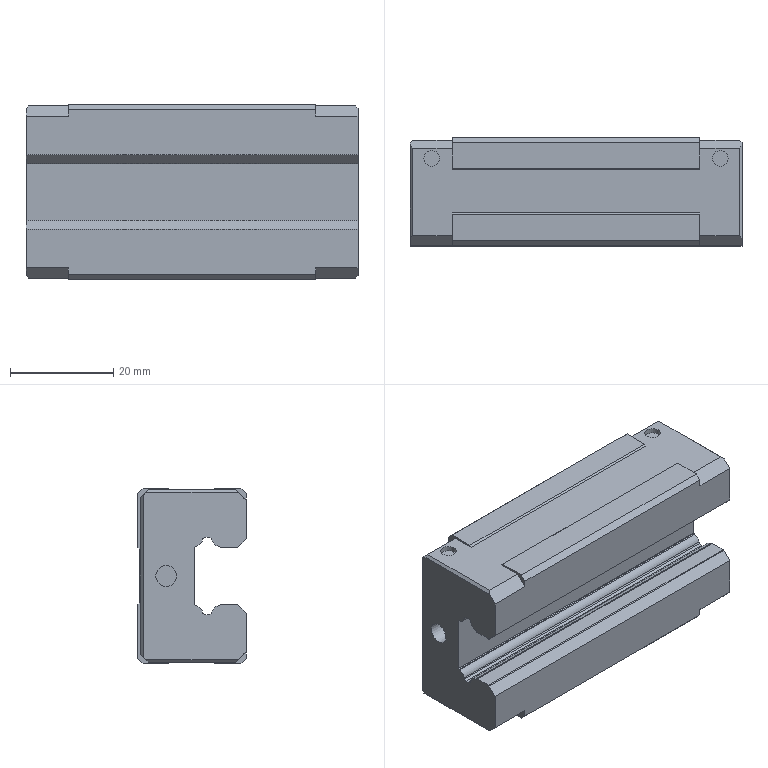Part | NX | 1 solid | 100 faces | box 64.4 x 21 x 34 mm | volume 36631 mm3 | plane 66 | cylinder 26 | cone 8 | commonest cylinder face diameters 0.6 x6 2.861 x4 3 x4 3.242 x4 0.398 x2 0.545 x2